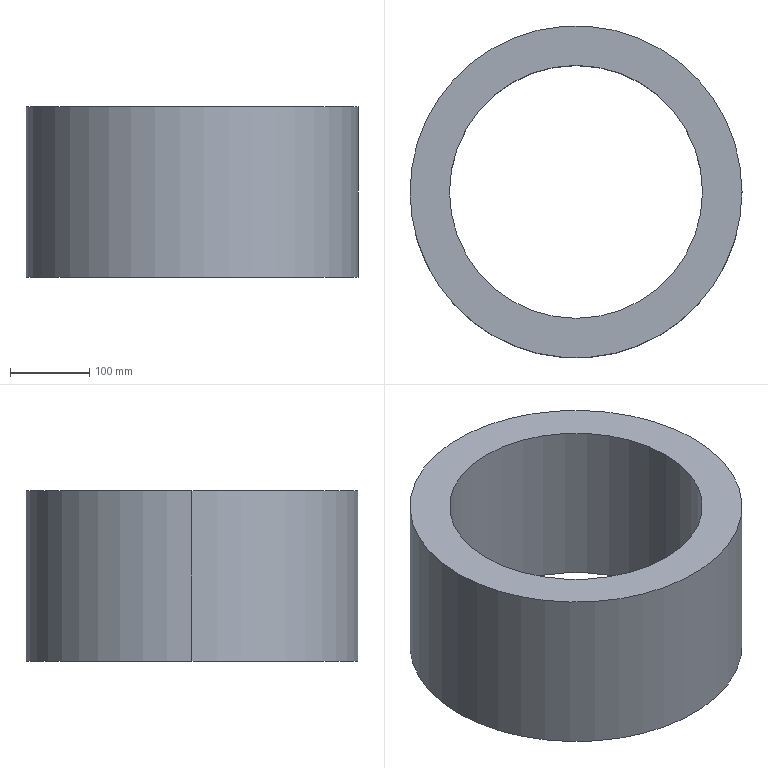Part | SolidWorks | features Extrusion 1, ICE 1 | 1 solid | 6 faces | box 420 x 420 x 216 mm | volume 12553804 mm3 | cylinder 4 | plane 2 | commonest cylinder face diameters 320 x2 420 x2
STEP:
#1=CARTESIAN_POINT('',(160.,0.,216.));
#2=VERTEX_POINT('',#1);
#3=CARTESIAN_POINT('',(-160.,0.,216.));
#4=VERTEX_POINT('',#3);
#5=CARTESIAN_POINT('',(0.,0.,216.));
#6=DIRECTION('',(0.,0.,-1.));
#7=DIRECTION('',(1.,0.,0.));
#8=AXIS2_PLACEMENT_3D('',#5,#6,#7);
#9=CIRCLE('',#8,160.);
#10=EDGE_CURVE('',#2,#4,#9,.T.);
#11=ORIENTED_EDGE('',*,*,#10,.F.);
#12=CARTESIAN_POINT('',(160.,0.,0.));
#13=VERTEX_POINT('',#12);
#14=CARTESIAN_POINT('',(160.,0.,250.));
#15=DIRECTION('',(0.,0.,-1.));
#16=VECTOR('',#15,1000.);
#17=LINE('',#14,#16);
#18=EDGE_CURVE('',#2,#13,#17,.T.);
#19=ORIENTED_EDGE('',*,*,#18,.T.);
#20=CARTESIAN_POINT('',(-160.,0.,0.));
#21=VERTEX_POINT('',#20);
#22=CARTESIAN_POINT('',(0.,0.,0.));
#23=DIRECTION('',(0.,0.,1.));
#24=DIRECTION('',(1.,0.,0.));
#25=AXIS2_PLACEMENT_3D('',#22,#23,#24);
#26=CIRCLE('',#25,160.);
#27=EDGE_CURVE('',#21,#13,#26,.T.);
#28=ORIENTED_EDGE('',*,*,#27,.F.);
#29=CARTESIAN_POINT('',(-160.,0.,250.));
#30=DIRECTION('',(0.,0.,-1.));
#31=VECTOR('',#30,1000.);
#32=LINE('',#29,#31);
#33=EDGE_CURVE('',#4,#21,#32,.T.);
#34=ORIENTED_EDGE('',*,*,#33,.F.);
#35=EDGE_LOOP('',(#11,#19,#28,#34));
#36=FACE_OUTER_BOUND('',#35,.T.);
#37=CARTESIAN_POINT('',(0.,0.,250.));
#38=DIRECTION('',(0.,0.,-1.));
#39=DIRECTION('',(-1.,0.,0.));
#40=AXIS2_PLACEMENT_3D('',#37,#38,#39);
#41=CYLINDRICAL_SURFACE('',#40,160.);
#42=ADVANCED_FACE('',(#36),#41,.F.);
#43=CARTESIAN_POINT('',(210.,0.,216.));
#44=VERTEX_POINT('',#43);
#45=CARTESIAN_POINT('',(-210.,0.,216.));
#46=VERTEX_POINT('',#45);
#47=CARTESIAN_POINT('',(0.,0.,216.));
#48=DIRECTION('',(0.,0.,1.));
#49=DIRECTION('',(1.,0.,0.));
#50=AXIS2_PLACEMENT_3D('',#47,#48,#49);
#51=CIRCLE('',#50,210.);
#52=EDGE_CURVE('',#44,#46,#51,.T.);
#53=ORIENTED_EDGE('',*,*,#52,.F.);
#54=CARTESIAN_POINT('',(210.,0.,0.));
#55=VERTEX_POINT('',#54);
#56=CARTESIAN_POINT('',(210.,0.,216.));
#57=DIRECTION('',(0.,0.,-1.));
#58=VECTOR('',#57,1000.);
#59=LINE('',#56,#58);
#60=EDGE_CURVE('',#44,#55,#59,.T.);
#61=ORIENTED_EDGE('',*,*,#60,.T.);
#62=CARTESIAN_POINT('',(-210.,0.,0.));
#63=VERTEX_POINT('',#62);
#64=CARTESIAN_POINT('',(0.,0.,0.));
#65=DIRECTION('',(0.,0.,1.));
#66=DIRECTION('',(1.,0.,0.));
#67=AXIS2_PLACEMENT_3D('',#64,#65,#66);
#68=CIRCLE('',#67,210.);
#69=EDGE_CURVE('',#55,#63,#68,.T.);
#70=ORIENTED_EDGE('',*,*,#69,.T.);
#71=CARTESIAN_POINT('',(-210.,0.,216.));
#72=DIRECTION('',(0.,0.,-1.));
#73=VECTOR('',#72,1000.);
#74=LINE('',#71,#73);
#75=EDGE_CURVE('',#46,#63,#74,.T.);
#76=ORIENTED_EDGE('',*,*,#75,.F.);
#77=EDGE_LOOP('',(#53,#61,#70,#76));
#78=FACE_OUTER_BOUND('',#77,.T.);
#79=CARTESIAN_POINT('',(0.,0.,216.));
#80=DIRECTION('',(0.,0.,-1.));
#81=DIRECTION('',(-1.,0.,0.));
#82=AXIS2_PLACEMENT_3D('',#79,#80,#81);
#83=CYLINDRICAL_SURFACE('',#82,210.);
#84=ADVANCED_FACE('',(#78),#83,.T.);
#85=ORIENTED_EDGE('',*,*,#60,.F.);
#86=CARTESIAN_POINT('',(0.,0.,216.));
#87=DIRECTION('',(0.,0.,1.));
#88=DIRECTION('',(1.,0.,0.));
#89=AXIS2_PLACEMENT_3D('',#86,#87,#88);
#90=CIRCLE('',#89,210.);
#91=EDGE_CURVE('',#46,#44,#90,.T.);
#92=ORIENTED_EDGE('',*,*,#91,.F.);
#93=ORIENTED_EDGE('',*,*,#75,.T.);
#94=CARTESIAN_POINT('',(0.,0.,0.));
#95=DIRECTION('',(0.,0.,1.));
#96=DIRECTION('',(1.,0.,0.));
#97=AXIS2_PLACEMENT_3D('',#94,#95,#96);
#98=CIRCLE('',#97,210.);
#99=EDGE_CURVE('',#63,#55,#98,.T.);
#100=ORIENTED_EDGE('',*,*,#99,.T.);
#101=EDGE_LOOP('',(#85,#92,#93,#100));
#102=FACE_OUTER_BOUND('',#101,.T.);
#103=CARTESIAN_POINT('',(0.,0.,216.));
#104=DIRECTION('',(0.,0.,-1.));
#105=DIRECTION('',(-1.,0.,0.));
#106=AXIS2_PLACEMENT_3D('',#103,#104,#105);
#107=CYLINDRICAL_SURFACE('',#106,210.);
#108=ADVANCED_FACE('',(#102),#107,.T.);
#109=CARTESIAN_POINT('',(0.,0.,216.));
#110=DIRECTION('',(0.,0.,-1.));
#111=DIRECTION('',(1.,0.,0.));
#112=AXIS2_PLACEMENT_3D('',#109,#110,#111);
#113=CIRCLE('',#112,160.);
#114=EDGE_CURVE('',#4,#2,#113,.T.);
#115=ORIENTED_EDGE('',*,*,#114,.T.);
#116=ORIENTED_EDGE('',*,*,#10,.T.);
#117=EDGE_LOOP('',(#115,#116));
#118=FACE_BOUND('',#117,.T.);
#119=ORIENTED_EDGE('',*,*,#91,.T.);
#120=ORIENTED_EDGE('',*,*,#52,.T.);
#121=EDGE_LOOP('',(#119,#120));
#122=FACE_OUTER_BOUND('',#121,.T.);
#123=CARTESIAN_POINT('',(0.,0.,216.));
#124=DIRECTION('',(0.,0.,1.));
#125=DIRECTION('',(1.,0.,0.));
#126=AXIS2_PLACEMENT_3D('',#123,#124,#125);
#127=PLANE('',#126);
#128=ADVANCED_FACE('',(#118,#122),#127,.T.);
#129=ORIENTED_EDGE('',*,*,#27,.T.);
#130=CARTESIAN_POINT('',(0.,0.,0.));
#131=DIRECTION('',(0.,0.,1.));
#132=DIRECTION('',(1.,0.,0.));
#133=AXIS2_PLACEMENT_3D('',#130,#131,#132);
#134=CIRCLE('',#133,160.);
#135=EDGE_CURVE('',#13,#21,#134,.T.);
#136=ORIENTED_EDGE('',*,*,#135,.T.);
#137=EDGE_LOOP('',(#129,#136));
#138=FACE_BOUND('',#137,.T.);
#139=ORIENTED_EDGE('',*,*,#99,.F.);
#140=ORIENTED_EDGE('',*,*,#69,.F.);
#141=EDGE_LOOP('',(#139,#140));
#142=FACE_OUTER_BOUND('',#141,.T.);
#143=CARTESIAN_POINT('',(0.,0.,0.));
#144=DIRECTION('',(0.,0.,1.));
#145=DIRECTION('',(1.,0.,0.));
#146=AXIS2_PLACEMENT_3D('',#143,#144,#145);
#147=PLANE('',#146);
#148=ADVANCED_FACE('',(#138,#142),#147,.F.);
#149=ORIENTED_EDGE('',*,*,#18,.F.);
#150=ORIENTED_EDGE('',*,*,#114,.F.);
#151=ORIENTED_EDGE('',*,*,#33,.T.);
#152=ORIENTED_EDGE('',*,*,#135,.F.);
#153=EDGE_LOOP('',(#149,#150,#151,#152));
#154=FACE_OUTER_BOUND('',#153,.T.);
#155=CARTESIAN_POINT('',(0.,0.,250.));
#156=DIRECTION('',(0.,0.,-1.));
#157=DIRECTION('',(-1.,0.,0.));
#158=AXIS2_PLACEMENT_3D('',#155,#156,#157);
#159=CYLINDRICAL_SURFACE('',#158,160.);
#160=ADVANCED_FACE('',(#154),#159,.F.);
#161=CLOSED_SHELL('',(#42,#84,#108,#128,#148,#160));
#162=MANIFOLD_SOLID_BREP('',#161);
#163=CARTESIAN_POINT('',(0.,0.,0.));
#164=DIRECTION('',(0.,0.,1.));
#165=DIRECTION('',(1.,0.,0.));
#166=AXIS2_PLACEMENT_3D('',#163,#164,#165);
#167=(LENGTH_UNIT()NAMED_UNIT(*)SI_UNIT(.MILLI.,.METRE.));
#168=UNCERTAINTY_MEASURE_WITH_UNIT(LENGTH_MEASURE(0.00001),#167,'','');
#169=(NAMED_UNIT(*)PLANE_ANGLE_UNIT()SI_UNIT($,.RADIAN.));
#170=(NAMED_UNIT(*)SI_UNIT($,.STERADIAN.)SOLID_ANGLE_UNIT());
#171=(GEOMETRIC_REPRESENTATION_CONTEXT(3)GLOBAL_UNCERTAINTY_ASSIGNED_CONTEXT((#168))GLOBAL_UNIT_ASSIGNED_CONTEXT((#167,#169,#170))REPRESENTATION_CONTEXT('',''));
#172=ADVANCED_BREP_SHAPE_REPRESENTATION('',(#162,#166),#171);